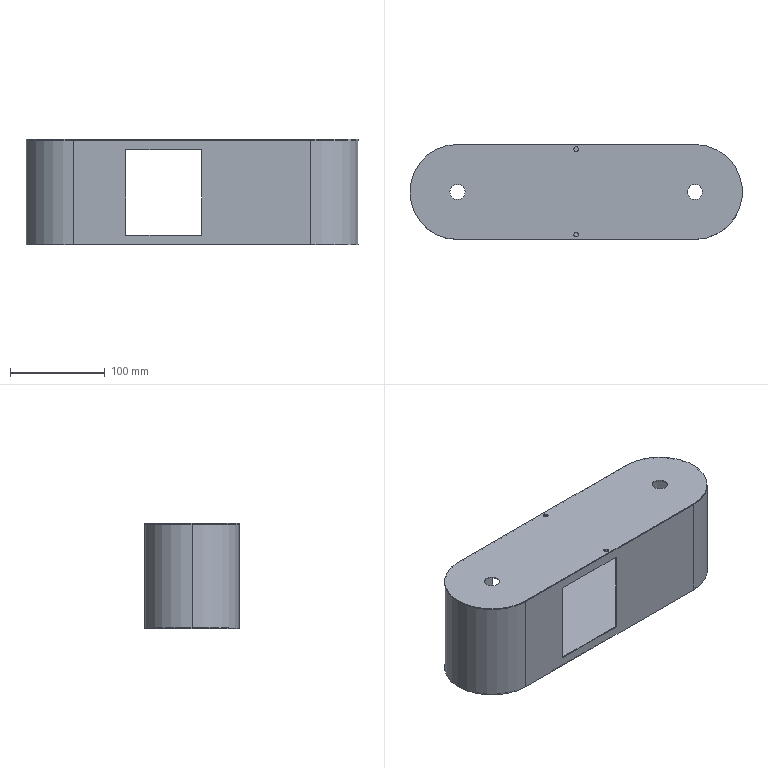Part | SolidWorks | features ICE 5, Extrusion 1, Shell 1 | 2 solids | 40 faces | box 350 x 100 x 111 mm | volume 133465 mm3 | cylinder 21 | plane 19 | commonest cylinder face diameters 16 x8 100 x6 5 x4 98 x3
STEP:
#1=CARTESIAN_POINT('',(122.5,-45.,110.));
#2=VERTEX_POINT('',#1);
#3=CARTESIAN_POINT('',(127.5,-45.,110.));
#4=VERTEX_POINT('',#3);
#5=CARTESIAN_POINT('',(125.,-45.,110.));
#6=DIRECTION('',(0.,0.,1.));
#7=DIRECTION('',(1.,0.,0.));
#8=AXIS2_PLACEMENT_3D('',#5,#6,#7);
#9=CIRCLE('',#8,2.5);
#10=EDGE_CURVE('',#2,#4,#9,.T.);
#11=ORIENTED_EDGE('',*,*,#10,.F.);
#12=CARTESIAN_POINT('',(122.5,-45.,111.));
#13=VERTEX_POINT('',#12);
#14=CARTESIAN_POINT('',(122.5,-45.,108.));
#15=DIRECTION('',(0.,0.,1.));
#16=VECTOR('',#15,1000.);
#17=LINE('',#14,#16);
#18=EDGE_CURVE('',#2,#13,#17,.T.);
#19=ORIENTED_EDGE('',*,*,#18,.T.);
#20=CARTESIAN_POINT('',(127.5,-45.,111.));
#21=VERTEX_POINT('',#20);
#22=CARTESIAN_POINT('',(125.,-45.,111.));
#23=DIRECTION('',(0.,0.,1.));
#24=DIRECTION('',(1.,0.,0.));
#25=AXIS2_PLACEMENT_3D('',#22,#23,#24);
#26=CIRCLE('',#25,2.5);
#27=EDGE_CURVE('',#13,#21,#26,.T.);
#28=ORIENTED_EDGE('',*,*,#27,.T.);
#29=CARTESIAN_POINT('',(127.5,-45.,108.));
#30=DIRECTION('',(0.,0.,1.));
#31=VECTOR('',#30,1000.);
#32=LINE('',#29,#31);
#33=EDGE_CURVE('',#4,#21,#32,.T.);
#34=ORIENTED_EDGE('',*,*,#33,.F.);
#35=EDGE_LOOP('',(#11,#19,#28,#34));
#36=FACE_OUTER_BOUND('',#35,.T.);
#37=CARTESIAN_POINT('',(125.,-45.,108.));
#38=DIRECTION('',(0.,0.,1.));
#39=DIRECTION('',(1.,0.,0.));
#40=AXIS2_PLACEMENT_3D('',#37,#38,#39);
#41=CYLINDRICAL_SURFACE('',#40,2.5);
#42=ADVANCED_FACE('',(#36),#41,.F.);
#43=CARTESIAN_POINT('',(122.5,45.,110.));
#44=VERTEX_POINT('',#43);
#45=CARTESIAN_POINT('',(127.5,45.,110.));
#46=VERTEX_POINT('',#45);
#47=CARTESIAN_POINT('',(125.,45.,110.));
#48=DIRECTION('',(0.,0.,1.));
#49=DIRECTION('',(1.,0.,0.));
#50=AXIS2_PLACEMENT_3D('',#47,#48,#49);
#51=CIRCLE('',#50,2.5);
#52=EDGE_CURVE('',#44,#46,#51,.T.);
#53=ORIENTED_EDGE('',*,*,#52,.F.);
#54=CARTESIAN_POINT('',(122.5,45.,111.));
#55=VERTEX_POINT('',#54);
#56=CARTESIAN_POINT('',(122.5,45.,108.));
#57=DIRECTION('',(0.,0.,1.));
#58=VECTOR('',#57,1000.);
#59=LINE('',#56,#58);
#60=EDGE_CURVE('',#44,#55,#59,.T.);
#61=ORIENTED_EDGE('',*,*,#60,.T.);
#62=CARTESIAN_POINT('',(127.5,45.,111.));
#63=VERTEX_POINT('',#62);
#64=CARTESIAN_POINT('',(125.,45.,111.));
#65=DIRECTION('',(0.,0.,1.));
#66=DIRECTION('',(1.,0.,0.));
#67=AXIS2_PLACEMENT_3D('',#64,#65,#66);
#68=CIRCLE('',#67,2.5);
#69=EDGE_CURVE('',#55,#63,#68,.T.);
#70=ORIENTED_EDGE('',*,*,#69,.T.);
#71=CARTESIAN_POINT('',(127.5,45.,108.));
#72=DIRECTION('',(0.,0.,1.));
#73=VECTOR('',#72,1000.);
#74=LINE('',#71,#73);
#75=EDGE_CURVE('',#46,#63,#74,.T.);
#76=ORIENTED_EDGE('',*,*,#75,.F.);
#77=EDGE_LOOP('',(#53,#61,#70,#76));
#78=FACE_OUTER_BOUND('',#77,.T.);
#79=CARTESIAN_POINT('',(125.,45.,108.));
#80=DIRECTION('',(0.,0.,1.));
#81=DIRECTION('',(1.,0.,0.));
#82=AXIS2_PLACEMENT_3D('',#79,#80,#81);
#83=CYLINDRICAL_SURFACE('',#82,2.5);
#84=ADVANCED_FACE('',(#78),#83,.F.);
#85=CARTESIAN_POINT('',(-8.,0.,110.));
#86=VERTEX_POINT('',#85);
#87=CARTESIAN_POINT('',(8.,0.,110.));
#88=VERTEX_POINT('',#87);
#89=CARTESIAN_POINT('',(0.,0.,110.));
#90=DIRECTION('',(0.,0.,1.));
#91=DIRECTION('',(1.,0.,0.));
#92=AXIS2_PLACEMENT_3D('',#89,#90,#91);
#93=CIRCLE('',#92,8.);
#94=EDGE_CURVE('',#86,#88,#93,.T.);
#95=ORIENTED_EDGE('',*,*,#94,.F.);
#96=CARTESIAN_POINT('',(-8.,0.,111.));
#97=VERTEX_POINT('',#96);
#98=CARTESIAN_POINT('',(-8.,0.,0.));
#99=DIRECTION('',(0.,0.,1.));
#100=VECTOR('',#99,1000.);
#101=LINE('',#98,#100);
#102=EDGE_CURVE('',#86,#97,#101,.T.);
#103=ORIENTED_EDGE('',*,*,#102,.T.);
#104=CARTESIAN_POINT('',(8.,0.,111.));
#105=VERTEX_POINT('',#104);
#106=CARTESIAN_POINT('',(0.,0.,111.));
#107=DIRECTION('',(0.,0.,1.));
#108=DIRECTION('',(1.,0.,0.));
#109=AXIS2_PLACEMENT_3D('',#106,#107,#108);
#110=CIRCLE('',#109,8.);
#111=EDGE_CURVE('',#97,#105,#110,.T.);
#112=ORIENTED_EDGE('',*,*,#111,.T.);
#113=CARTESIAN_POINT('',(8.,0.,0.));
#114=DIRECTION('',(0.,0.,1.));
#115=VECTOR('',#114,1000.);
#116=LINE('',#113,#115);
#117=EDGE_CURVE('',#88,#105,#116,.T.);
#118=ORIENTED_EDGE('',*,*,#117,.F.);
#119=EDGE_LOOP('',(#95,#103,#112,#118));
#120=FACE_OUTER_BOUND('',#119,.T.);
#121=CARTESIAN_POINT('',(0.,0.,0.));
#122=DIRECTION('',(0.,0.,1.));
#123=DIRECTION('',(1.,0.,0.));
#124=AXIS2_PLACEMENT_3D('',#121,#122,#123);
#125=CYLINDRICAL_SURFACE('',#124,8.);
#126=ADVANCED_FACE('',(#120),#125,.F.);
#127=CARTESIAN_POINT('',(242.,0.,110.));
#128=VERTEX_POINT('',#127);
#129=CARTESIAN_POINT('',(258.,0.,110.));
#130=VERTEX_POINT('',#129);
#131=CARTESIAN_POINT('',(250.,0.,110.));
#132=DIRECTION('',(0.,0.,1.));
#133=DIRECTION('',(1.,0.,0.));
#134=AXIS2_PLACEMENT_3D('',#131,#132,#133);
#135=CIRCLE('',#134,8.);
#136=EDGE_CURVE('',#128,#130,#135,.T.);
#137=ORIENTED_EDGE('',*,*,#136,.F.);
#138=CARTESIAN_POINT('',(242.,0.,111.));
#139=VERTEX_POINT('',#138);
#140=CARTESIAN_POINT('',(242.,0.,0.));
#141=DIRECTION('',(0.,0.,1.));
#142=VECTOR('',#141,1000.);
#143=LINE('',#140,#142);
#144=EDGE_CURVE('',#128,#139,#143,.T.);
#145=ORIENTED_EDGE('',*,*,#144,.T.);
#146=CARTESIAN_POINT('',(258.,0.,111.));
#147=VERTEX_POINT('',#146);
#148=CARTESIAN_POINT('',(250.,0.,111.));
#149=DIRECTION('',(0.,0.,1.));
#150=DIRECTION('',(1.,0.,0.));
#151=AXIS2_PLACEMENT_3D('',#148,#149,#150);
#152=CIRCLE('',#151,8.);
#153=EDGE_CURVE('',#139,#147,#152,.T.);
#154=ORIENTED_EDGE('',*,*,#153,.T.);
#155=CARTESIAN_POINT('',(258.,0.,0.));
#156=DIRECTION('',(0.,0.,1.));
#157=VECTOR('',#156,1000.);
#158=LINE('',#155,#157);
#159=EDGE_CURVE('',#130,#147,#158,.T.);
#160=ORIENTED_EDGE('',*,*,#159,.F.);
#161=EDGE_LOOP('',(#137,#145,#154,#160));
#162=FACE_OUTER_BOUND('',#161,.T.);
#163=CARTESIAN_POINT('',(250.,0.,0.));
#164=DIRECTION('',(0.,0.,1.));
#165=DIRECTION('',(1.,0.,0.));
#166=AXIS2_PLACEMENT_3D('',#163,#164,#165);
#167=CYLINDRICAL_SURFACE('',#166,8.);
#168=ADVANCED_FACE('',(#162),#167,.F.);
#169=CARTESIAN_POINT('',(-50.,0.,111.));
#170=VERTEX_POINT('',#169);
#171=CARTESIAN_POINT('',(0.,-50.,111.));
#172=VERTEX_POINT('',#171);
#173=CARTESIAN_POINT('',(0.,0.,111.));
#174=DIRECTION('',(0.,0.,1.));
#175=DIRECTION('',(1.,0.,0.));
#176=AXIS2_PLACEMENT_3D('',#173,#174,#175);
#177=CIRCLE('',#176,50.);
#178=EDGE_CURVE('',#170,#172,#177,.T.);
#179=ORIENTED_EDGE('',*,*,#178,.F.);
#180=CARTESIAN_POINT('',(-50.,0.,110.));
#181=VERTEX_POINT('',#180);
#182=CARTESIAN_POINT('',(-50.,0.,111.));
#183=DIRECTION('',(0.,0.,-1.));
#184=VECTOR('',#183,1000.);
#185=LINE('',#182,#184);
#186=EDGE_CURVE('',#170,#181,#185,.T.);
#187=ORIENTED_EDGE('',*,*,#186,.T.);
#188=CARTESIAN_POINT('',(0.,-50.,110.));
#189=VERTEX_POINT('',#188);
#190=CARTESIAN_POINT('',(0.,0.,110.));
#191=DIRECTION('',(0.,0.,1.));
#192=DIRECTION('',(1.,0.,0.));
#193=AXIS2_PLACEMENT_3D('',#190,#191,#192);
#194=CIRCLE('',#193,50.);
#195=EDGE_CURVE('',#181,#189,#194,.T.);
#196=ORIENTED_EDGE('',*,*,#195,.T.);
#197=CARTESIAN_POINT('',(0.,-50.,111.));
#198=DIRECTION('',(0.,0.,-1.));
#199=VECTOR('',#198,1000.);
#200=LINE('',#197,#199);
#201=EDGE_CURVE('',#172,#189,#200,.T.);
#202=ORIENTED_EDGE('',*,*,#201,.F.);
#203=EDGE_LOOP('',(#179,#187,#196,#202));
#204=FACE_OUTER_BOUND('',#203,.T.);
#205=CARTESIAN_POINT('',(0.,0.,111.));
#206=DIRECTION('',(0.,0.,-1.));
#207=DIRECTION('',(-1.,0.,0.));
#208=AXIS2_PLACEMENT_3D('',#205,#206,#207);
#209=CYLINDRICAL_SURFACE('',#208,50.);
#210=ADVANCED_FACE('',(#204),#209,.T.);
#211=CARTESIAN_POINT('',(250.,-50.,110.));
#212=VERTEX_POINT('',#211);
#213=CARTESIAN_POINT('',(250.,50.,110.));
#214=VERTEX_POINT('',#213);
#215=CARTESIAN_POINT('',(250.,0.,110.));
#216=DIRECTION('',(0.,0.,1.));
#217=DIRECTION('',(1.,0.,0.));
#218=AXIS2_PLACEMENT_3D('',#215,#216,#217);
#219=CIRCLE('',#218,50.);
#220=EDGE_CURVE('',#212,#214,#219,.T.);
#221=ORIENTED_EDGE('',*,*,#220,.T.);
#222=CARTESIAN_POINT('',(250.,50.,111.));
#223=VERTEX_POINT('',#222);
#224=CARTESIAN_POINT('',(250.,50.,111.));
#225=DIRECTION('',(0.,0.,-1.));
#226=VECTOR('',#225,1000.);
#227=LINE('',#224,#226);
#228=EDGE_CURVE('',#223,#214,#227,.T.);
#229=ORIENTED_EDGE('',*,*,#228,.F.);
#230=CARTESIAN_POINT('',(250.,-50.,111.));
#231=VERTEX_POINT('',#230);
#232=CARTESIAN_POINT('',(250.,0.,111.));
#233=DIRECTION('',(0.,0.,1.));
#234=DIRECTION('',(1.,0.,0.));
#235=AXIS2_PLACEMENT_3D('',#232,#233,#234);
#236=CIRCLE('',#235,50.);
#237=EDGE_CURVE('',#231,#223,#236,.T.);
#238=ORIENTED_EDGE('',*,*,#237,.F.);
#239=CARTESIAN_POINT('',(250.,-50.,111.));
#240=DIRECTION('',(0.,0.,-1.));
#241=VECTOR('',#240,1000.);
#242=LINE('',#239,#241);
#243=EDGE_CURVE('',#231,#212,#242,.T.);
#244=ORIENTED_EDGE('',*,*,#243,.T.);
#245=EDGE_LOOP('',(#221,#229,#238,#244));
#246=FACE_OUTER_BOUND('',#245,.T.);
#247=CARTESIAN_POINT('',(250.,0.,111.));
#248=DIRECTION('',(0.,0.,-1.));
#249=DIRECTION('',(-1.,0.,0.));
#250=AXIS2_PLACEMENT_3D('',#247,#248,#249);
#251=CYLINDRICAL_SURFACE('',#250,50.);
#252=ADVANCED_FACE('',(#246),#251,.T.);
#253=CARTESIAN_POINT('',(0.,50.,110.));
#254=VERTEX_POINT('',#253);
#255=CARTESIAN_POINT('',(250.,50.,110.));
#256=DIRECTION('',(-1.,0.,0.));
#257=VECTOR('',#256,1000.);
#258=LINE('',#255,#257);
#259=EDGE_CURVE('',#214,#254,#258,.T.);
#260=ORIENTED_EDGE('',*,*,#259,.T.);
#261=CARTESIAN_POINT('',(0.,50.,111.));
#262=VERTEX_POINT('',#261);
#263=CARTESIAN_POINT('',(0.,50.,111.));
#264=DIRECTION('',(0.,0.,-1.));
#265=VECTOR('',#264,1000.);
#266=LINE('',#263,#265);
#267=EDGE_CURVE('',#262,#254,#266,.T.);
#268=ORIENTED_EDGE('',*,*,#267,.F.);
#269=CARTESIAN_POINT('',(250.,50.,111.));
#270=DIRECTION('',(-1.,0.,0.));
#271=VECTOR('',#270,1000.);
#272=LINE('',#269,#271);
#273=EDGE_CURVE('',#223,#262,#272,.T.);
#274=ORIENTED_EDGE('',*,*,#273,.F.);
#275=ORIENTED_EDGE('',*,*,#228,.T.);
#276=EDGE_LOOP('',(#260,#268,#274,#275));
#277=FACE_OUTER_BOUND('',#276,.T.);
#278=CARTESIAN_POINT('',(250.,50.,111.));
#279=DIRECTION('',(0.,-1.,0.));
#280=DIRECTION('',(0.,0.,-1.));
#281=AXIS2_PLACEMENT_3D('',#278,#279,#280);
#282=PLANE('',#281);
#283=ADVANCED_FACE('',(#277),#282,.F.);
#284=ORIENTED_EDGE('',*,*,#186,.F.);
#285=CARTESIAN_POINT('',(0.,0.,111.));
#286=DIRECTION('',(0.,0.,1.));
#287=DIRECTION('',(1.,0.,0.));
#288=AXIS2_PLACEMENT_3D('',#285,#286,#287);
#289=CIRCLE('',#288,50.);
#290=EDGE_CURVE('',#262,#170,#289,.T.);
#291=ORIENTED_EDGE('',*,*,#290,.F.);
#292=ORIENTED_EDGE('',*,*,#267,.T.);
#293=CARTESIAN_POINT('',(0.,0.,110.));
#294=DIRECTION('',(0.,0.,1.));
#295=DIRECTION('',(1.,0.,0.));
#296=AXIS2_PLACEMENT_3D('',#293,#294,#295);
#297=CIRCLE('',#296,50.);
#298=EDGE_CURVE('',#254,#181,#297,.T.);
#299=ORIENTED_EDGE('',*,*,#298,.T.);
#300=EDGE_LOOP('',(#284,#291,#292,#299));
#301=FACE_OUTER_BOUND('',#300,.T.);
#302=CARTESIAN_POINT('',(0.,0.,111.));
#303=DIRECTION('',(0.,0.,-1.));
#304=DIRECTION('',(-1.,0.,0.));
#305=AXIS2_PLACEMENT_3D('',#302,#303,#304);
#306=CYLINDRICAL_SURFACE('',#305,50.);
#307=ADVANCED_FACE('',(#301),#306,.T.);
#308=CARTESIAN_POINT('',(0.,-50.,110.));
#309=DIRECTION('',(1.,0.,0.));
#310=VECTOR('',#309,1000.);
#311=LINE('',#308,#310);
#312=EDGE_CURVE('',#189,#212,#311,.T.);
#313=ORIENTED_EDGE('',*,*,#312,.T.);
#314=ORIENTED_EDGE('',*,*,#243,.F.);
#315=CARTESIAN_POINT('',(0.,-50.,111.));
#316=DIRECTION('',(1.,0.,0.));
#317=VECTOR('',#316,1000.);
#318=LINE('',#315,#317);
#319=EDGE_CURVE('',#172,#231,#318,.T.);
#320=ORIENTED_EDGE('',*,*,#319,.F.);
#321=ORIENTED_EDGE('',*,*,#201,.T.);
#322=EDGE_LOOP('',(#313,#314,#320,#321));
#323=FACE_OUTER_BOUND('',#322,.T.);
#324=CARTESIAN_POINT('',(0.,-50.,111.));
#325=DIRECTION('',(0.,1.,0.));
#326=DIRECTION('',(0.,0.,1.));
#327=AXIS2_PLACEMENT_3D('',#324,#325,#326);
#328=PLANE('',#327);
#329=ADVANCED_FACE('',(#323),#328,.F.);
#330=CARTESIAN_POINT('',(125.,-45.,111.));
#331=DIRECTION('',(0.,0.,1.));
#332=DIRECTION('',(1.,0.,0.));
#333=AXIS2_PLACEMENT_3D('',#330,#331,#332);
#334=CIRCLE('',#333,2.5);
#335=EDGE_CURVE('',#21,#13,#334,.T.);
#336=ORIENTED_EDGE('',*,*,#335,.F.);
#337=ORIENTED_EDGE('',*,*,#27,.F.);
#338=EDGE_LOOP('',(#336,#337));
#339=FACE_BOUND('',#338,.T.);
#340=CARTESIAN_POINT('',(125.,45.,111.));
#341=DIRECTION('',(0.,0.,1.));
#342=DIRECTION('',(1.,0.,0.));
#343=AXIS2_PLACEMENT_3D('',#340,#341,#342);
#344=CIRCLE('',#343,2.5);
#345=EDGE_CURVE('',#63,#55,#344,.T.);
#346=ORIENTED_EDGE('',*,*,#345,.F.);
#347=ORIENTED_EDGE('',*,*,#69,.F.);
#348=EDGE_LOOP('',(#346,#347));
#349=FACE_BOUND('',#348,.T.);
#350=CARTESIAN_POINT('',(0.,0.,111.));
#351=DIRECTION('',(0.,0.,1.));
#352=DIRECTION('',(1.,0.,0.));
#353=AXIS2_PLACEMENT_3D('',#350,#351,#352);
#354=CIRCLE('',#353,8.);
#355=EDGE_CURVE('',#105,#97,#354,.T.);
#356=ORIENTED_EDGE('',*,*,#355,.F.);
#357=ORIENTED_EDGE('',*,*,#111,.F.);
#358=EDGE_LOOP('',(#356,#357));
#359=FACE_BOUND('',#358,.T.);
#360=CARTESIAN_POINT('',(250.,0.,111.));
#361=DIRECTION('',(0.,0.,1.));
#362=DIRECTION('',(1.,0.,0.));
#363=AXIS2_PLACEMENT_3D('',#360,#361,#362);
#364=CIRCLE('',#363,8.);
#365=EDGE_CURVE('',#147,#139,#364,.T.);
#366=ORIENTED_EDGE('',*,*,#365,.F.);
#367=ORIENTED_EDGE('',*,*,#153,.F.);
#368=EDGE_LOOP('',(#366,#367));
#369=FACE_BOUND('',#368,.T.);
#370=ORIENTED_EDGE('',*,*,#237,.T.);
#371=ORIENTED_EDGE('',*,*,#273,.T.);
#372=ORIENTED_EDGE('',*,*,#290,.T.);
#373=ORIENTED_EDGE('',*,*,#178,.T.);
#374=ORIENTED_EDGE('',*,*,#319,.T.);
#375=EDGE_LOOP('',(#370,#371,#372,#373,#374));
#376=FACE_OUTER_BOUND('',#375,.T.);
#377=CARTESIAN_POINT('',(250.,0.,111.));
#378=DIRECTION('',(0.,0.,1.));
#379=DIRECTION('',(1.,0.,0.));
#380=AXIS2_PLACEMENT_3D('',#377,#378,#379);
#381=PLANE('',#380);
#382=ADVANCED_FACE('',(#339,#349,#359,#369,#376),#381,.T.);
#383=CARTESIAN_POINT('',(125.,-45.,110.));
#384=DIRECTION('',(0.,0.,1.));
#385=DIRECTION('',(1.,0.,0.));
#386=AXIS2_PLACEMENT_3D('',#383,#384,#385);
#387=CIRCLE('',#386,2.5);
#388=EDGE_CURVE('',#4,#2,#387,.T.);
#389=ORIENTED_EDGE('',*,*,#388,.T.);
#390=ORIENTED_EDGE('',*,*,#10,.T.);
#391=EDGE_LOOP('',(#389,#390));
#392=FACE_BOUND('',#391,.T.);
#393=CARTESIAN_POINT('',(125.,45.,110.));
#394=DIRECTION('',(0.,0.,1.));
#395=DIRECTION('',(1.,0.,0.));
#396=AXIS2_PLACEMENT_3D('',#393,#394,#395);
#397=CIRCLE('',#396,2.5);
#398=EDGE_CURVE('',#46,#44,#397,.T.);
#399=ORIENTED_EDGE('',*,*,#398,.T.);
#400=ORIENTED_EDGE('',*,*,#52,.T.);
#401=EDGE_LOOP('',(#399,#400));
#402=FACE_BOUND('',#401,.T.);
#403=CARTESIAN_POINT('',(0.,0.,110.));
#404=DIRECTION('',(0.,0.,1.));
#405=DIRECTION('',(1.,0.,0.));
#406=AXIS2_PLACEMENT_3D('',#403,#404,#405);
#407=CIRCLE('',#406,8.);
#408=EDGE_CURVE('',#88,#86,#407,.T.);
#409=ORIENTED_EDGE('',*,*,#408,.T.);
#410=ORIENTED_EDGE('',*,*,#94,.T.);
#411=EDGE_LOOP('',(#409,#410));
#412=FACE_BOUND('',#411,.T.);
#413=CARTESIAN_POINT('',(250.,0.,110.));
#414=DIRECTION('',(0.,0.,1.));
#415=DIRECTION('',(1.,0.,0.));
#416=AXIS2_PLACEMENT_3D('',#413,#414,#415);
#417=CIRCLE('',#416,8.);
#418=EDGE_CURVE('',#130,#128,#417,.T.);
#419=ORIENTED_EDGE('',*,*,#418,.T.);
#420=ORIENTED_EDGE('',*,*,#136,.T.);
#421=EDGE_LOOP('',(#419,#420));
#422=FACE_BOUND('',#421,.T.);
#423=ORIENTED_EDGE('',*,*,#220,.F.);
#424=ORIENTED_EDGE('',*,*,#312,.F.);
#425=ORIENTED_EDGE('',*,*,#195,.F.);
#426=ORIENTED_EDGE('',*,*,#298,.F.);
#427=ORIENTED_EDGE('',*,*,#259,.F.);
#428=EDGE_LOOP('',(#423,#424,#425,#426,#427));
#429=FACE_OUTER_BOUND('',#428,.T.);
#430=CARTESIAN_POINT('',(250.,0.,110.));
#431=DIRECTION('',(0.,0.,1.));
#432=DIRECTION('',(1.,0.,0.));
#433=AXIS2_PLACEMENT_3D('',#430,#431,#432);
#434=PLANE('',#433);
#435=ADVANCED_FACE('',(#392,#402,#412,#422,#429),#434,.F.);
#436=ORIENTED_EDGE('',*,*,#144,.F.);
#437=ORIENTED_EDGE('',*,*,#418,.F.);
#438=ORIENTED_EDGE('',*,*,#159,.T.);
#439=ORIENTED_EDGE('',*,*,#365,.T.);
#440=EDGE_LOOP('',(#436,#437,#438,#439));
#441=FACE_OUTER_BOUND('',#440,.T.);
#442=CARTESIAN_POINT('',(250.,0.,0.));
#443=DIRECTION('',(0.,0.,1.));
#444=DIRECTION('',(1.,0.,0.));
#445=AXIS2_PLACEMENT_3D('',#442,#443,#444);
#446=CYLINDRICAL_SURFACE('',#445,8.);
#447=ADVANCED_FACE('',(#441),#446,.F.);
#448=ORIENTED_EDGE('',*,*,#102,.F.);
#449=ORIENTED_EDGE('',*,*,#408,.F.);
#450=ORIENTED_EDGE('',*,*,#117,.T.);
#451=ORIENTED_EDGE('',*,*,#355,.T.);
#452=EDGE_LOOP('',(#448,#449,#450,#451));
#453=FACE_OUTER_BOUND('',#452,.T.);
#454=CARTESIAN_POINT('',(0.,0.,0.));
#455=DIRECTION('',(0.,0.,1.));
#456=DIRECTION('',(1.,0.,0.));
#457=AXIS2_PLACEMENT_3D('',#454,#455,#456);
#458=CYLINDRICAL_SURFACE('',#457,8.);
#459=ADVANCED_FACE('',(#453),#458,.F.);
#460=ORIENTED_EDGE('',*,*,#60,.F.);
#461=ORIENTED_EDGE('',*,*,#398,.F.);
#462=ORIENTED_EDGE('',*,*,#75,.T.);
#463=ORIENTED_EDGE('',*,*,#345,.T.);
#464=EDGE_LOOP('',(#460,#461,#462,#463));
#465=FACE_OUTER_BOUND('',#464,.T.);
#466=CARTESIAN_POINT('',(125.,45.,108.));
#467=DIRECTION('',(0.,0.,1.));
#468=DIRECTION('',(1.,0.,0.));
#469=AXIS2_PLACEMENT_3D('',#466,#467,#468);
#470=CYLINDRICAL_SURFACE('',#469,2.5);
#471=ADVANCED_FACE('',(#465),#470,.F.);
#472=ORIENTED_EDGE('',*,*,#18,.F.);
#473=ORIENTED_EDGE('',*,*,#388,.F.);
#474=ORIENTED_EDGE('',*,*,#33,.T.);
#475=ORIENTED_EDGE('',*,*,#335,.T.);
#476=EDGE_LOOP('',(#472,#473,#474,#475));
#477=FACE_OUTER_BOUND('',#476,.T.);
#478=CARTESIAN_POINT('',(125.,-45.,108.));
#479=DIRECTION('',(0.,0.,1.));
#480=DIRECTION('',(1.,0.,0.));
#481=AXIS2_PLACEMENT_3D('',#478,#479,#480);
#482=CYLINDRICAL_SURFACE('',#481,2.5);
#483=ADVANCED_FACE('',(#477),#482,.F.);
#484=CLOSED_SHELL('',(#42,#84,#126,#168,#210,#252,#283,#307,#329,#382,#435,#447,#459,#471,#483));
#485=MANIFOLD_SOLID_BREP('',#484);
#486=CARTESIAN_POINT('',(-8.,0.,0.));
#487=VERTEX_POINT('',#486);
#488=CARTESIAN_POINT('',(8.,0.,0.));
#489=VERTEX_POINT('',#488);
#490=CARTESIAN_POINT('',(0.,0.,0.));
#491=DIRECTION('',(0.,0.,1.));
#492=DIRECTION('',(1.,0.,0.));
#493=AXIS2_PLACEMENT_3D('',#490,#491,#492);
#494=CIRCLE('',#493,8.);
#495=EDGE_CURVE('',#487,#489,#494,.T.);
#496=ORIENTED_EDGE('',*,*,#495,.F.);
#497=CARTESIAN_POINT('',(-8.,0.,1.));
#498=VERTEX_POINT('',#497);
#499=CARTESIAN_POINT('',(-8.,0.,0.));
#500=DIRECTION('',(0.,0.,1.));
#501=VECTOR('',#500,1000.);
#502=LINE('',#499,#501);
#503=EDGE_CURVE('',#487,#498,#502,.T.);
#504=ORIENTED_EDGE('',*,*,#503,.T.);
#505=CARTESIAN_POINT('',(8.,0.,1.));
#506=VERTEX_POINT('',#505);
#507=CARTESIAN_POINT('',(0.,0.,1.));
#508=DIRECTION('',(0.,0.,1.));
#509=DIRECTION('',(1.,0.,0.));
#510=AXIS2_PLACEMENT_3D('',#507,#508,#509);
#511=CIRCLE('',#510,8.);
#512=EDGE_CURVE('',#498,#506,#511,.T.);
#513=ORIENTED_EDGE('',*,*,#512,.T.);
#514=CARTESIAN_POINT('',(8.,0.,0.));
#515=DIRECTION('',(0.,0.,1.));
#516=VECTOR('',#515,1000.);
#517=LINE('',#514,#516);
#518=EDGE_CURVE('',#489,#506,#517,.T.);
#519=ORIENTED_EDGE('',*,*,#518,.F.);
#520=EDGE_LOOP('',(#496,#504,#513,#519));
#521=FACE_OUTER_BOUND('',#520,.T.);
#522=CARTESIAN_POINT('',(0.,0.,0.));
#523=DIRECTION('',(0.,0.,1.));
#524=DIRECTION('',(1.,0.,0.));
#525=AXIS2_PLACEMENT_3D('',#522,#523,#524);
#526=CYLINDRICAL_SURFACE('',#525,8.);
#527=ADVANCED_FACE('',(#521),#526,.F.);
#528=CARTESIAN_POINT('',(242.,0.,0.));
#529=VERTEX_POINT('',#528);
#530=CARTESIAN_POINT('',(258.,0.,0.));
#531=VERTEX_POINT('',#530);
#532=CARTESIAN_POINT('',(250.,0.,0.));
#533=DIRECTION('',(0.,0.,1.));
#534=DIRECTION('',(1.,0.,0.));
#535=AXIS2_PLACEMENT_3D('',#532,#533,#534);
#536=CIRCLE('',#535,8.);
#537=EDGE_CURVE('',#529,#531,#536,.T.);
#538=ORIENTED_EDGE('',*,*,#537,.F.);
#539=CARTESIAN_POINT('',(242.,0.,1.));
#540=VERTEX_POINT('',#539);
#541=CARTESIAN_POINT('',(242.,0.,0.));
#542=DIRECTION('',(0.,0.,1.));
#543=VECTOR('',#542,1000.);
#544=LINE('',#541,#543);
#545=EDGE_CURVE('',#529,#540,#544,.T.);
#546=ORIENTED_EDGE('',*,*,#545,.T.);
#547=CARTESIAN_POINT('',(258.,0.,1.));
#548=VERTEX_POINT('',#547);
#549=CARTESIAN_POINT('',(250.,0.,1.));
#550=DIRECTION('',(0.,0.,1.));
#551=DIRECTION('',(1.,0.,0.));
#552=AXIS2_PLACEMENT_3D('',#549,#550,#551);
#553=CIRCLE('',#552,8.);
#554=EDGE_CURVE('',#540,#548,#553,.T.);
#555=ORIENTED_EDGE('',*,*,#554,.T.);
#556=CARTESIAN_POINT('',(258.,0.,0.));
#557=DIRECTION('',(0.,0.,1.));
#558=VECTOR('',#557,1000.);
#559=LINE('',#556,#558);
#560=EDGE_CURVE('',#531,#548,#559,.T.);
#561=ORIENTED_EDGE('',*,*,#560,.F.);
#562=EDGE_LOOP('',(#538,#546,#555,#561));
#563=FACE_OUTER_BOUND('',#562,.T.);
#564=CARTESIAN_POINT('',(250.,0.,0.));
#565=DIRECTION('',(0.,0.,1.));
#566=DIRECTION('',(1.,0.,0.));
#567=AXIS2_PLACEMENT_3D('',#564,#565,#566);
#568=CYLINDRICAL_SURFACE('',#567,8.);
#569=ADVANCED_FACE('',(#563),#568,.F.);
#570=CARTESIAN_POINT('',(0.,49.,110.));
#571=VERTEX_POINT('',#570);
#572=CARTESIAN_POINT('',(-49.,0.,110.));
#573=VERTEX_POINT('',#572);
#574=CARTESIAN_POINT('',(0.,0.,110.));
#575=DIRECTION('',(0.,0.,1.));
#576=DIRECTION('',(1.,0.,0.));
#577=AXIS2_PLACEMENT_3D('',#574,#575,#576);
#578=CIRCLE('',#577,49.);
#579=EDGE_CURVE('',#571,#573,#578,.T.);
#580=ORIENTED_EDGE('',*,*,#579,.T.);
#581=CARTESIAN_POINT('',(-49.,0.,1.));
#582=VERTEX_POINT('',#581);
#583=CARTESIAN_POINT('',(-49.,0.,110.));
#584=DIRECTION('',(0.,0.,-1.));
#585=VECTOR('',#584,1000.);
#586=LINE('',#583,#585);
#587=EDGE_CURVE('',#573,#582,#586,.T.);
#588=ORIENTED_EDGE('',*,*,#587,.T.);
#589=CARTESIAN_POINT('',(0.,49.,1.));
#590=VERTEX_POINT('',#589);
#591=CARTESIAN_POINT('',(0.,0.,1.));
#592=DIRECTION('',(0.,0.,1.));
#593=DIRECTION('',(1.,0.,0.));
#594=AXIS2_PLACEMENT_3D('',#591,#592,#593);
#595=CIRCLE('',#594,49.);
#596=EDGE_CURVE('',#590,#582,#595,.T.);
#597=ORIENTED_EDGE('',*,*,#596,.F.);
#598=CARTESIAN_POINT('',(0.,49.,110.));
#599=DIRECTION('',(0.,0.,-1.));
#600=VECTOR('',#599,1000.);
#601=LINE('',#598,#600);
#602=EDGE_CURVE('',#571,#590,#601,.T.);
#603=ORIENTED_EDGE('',*,*,#602,.F.);
#604=EDGE_LOOP('',(#580,#588,#597,#603));
#605=FACE_OUTER_BOUND('',#604,.T.);
#606=CARTESIAN_POINT('',(0.,0.,110.));
#607=DIRECTION('',(0.,0.,-1.));
#608=DIRECTION('',(-1.,0.,0.));
#609=AXIS2_PLACEMENT_3D('',#606,#607,#608);
#610=CYLINDRICAL_SURFACE('',#609,49.);
#611=ADVANCED_FACE('',(#605),#610,.F.);
#612=CARTESIAN_POINT('',(-50.,0.,110.));
#613=VERTEX_POINT('',#612);
#614=CARTESIAN_POINT('',(0.,-50.,110.));
#615=VERTEX_POINT('',#614);
#616=CARTESIAN_POINT('',(0.,0.,110.));
#617=DIRECTION('',(0.,0.,1.));
#618=DIRECTION('',(1.,0.,0.));
#619=AXIS2_PLACEMENT_3D('',#616,#617,#618);
#620=CIRCLE('',#619,50.);
#621=EDGE_CURVE('',#613,#615,#620,.T.);
#622=ORIENTED_EDGE('',*,*,#621,.F.);
#623=CARTESIAN_POINT('',(-50.,0.,0.));
#624=VERTEX_POINT('',#623);
#625=CARTESIAN_POINT('',(-50.,0.,110.));
#626=DIRECTION('',(0.,0.,-1.));
#627=VECTOR('',#626,1000.);
#628=LINE('',#625,#627);
#629=EDGE_CURVE('',#613,#624,#628,.T.);
#630=ORIENTED_EDGE('',*,*,#629,.T.);
#631=CARTESIAN_POINT('',(0.,-50.,0.));
#632=VERTEX_POINT('',#631);
#633=CARTESIAN_POINT('',(0.,0.,0.));
#634=DIRECTION('',(0.,0.,1.));
#635=DIRECTION('',(1.,0.,0.));
#636=AXIS2_PLACEMENT_3D('',#633,#634,#635);
#637=CIRCLE('',#636,50.);
#638=EDGE_CURVE('',#624,#632,#637,.T.);
#639=ORIENTED_EDGE('',*,*,#638,.T.);
#640=CARTESIAN_POINT('',(0.,-50.,110.));
#641=DIRECTION('',(0.,0.,-1.));
#642=VECTOR('',#641,1000.);
#643=LINE('',#640,#642);
#644=EDGE_CURVE('',#615,#632,#643,.T.);
#645=ORIENTED_EDGE('',*,*,#644,.F.);
#646=EDGE_LOOP('',(#622,#630,#639,#645));
#647=FACE_OUTER_BOUND('',#646,.T.);
#648=CARTESIAN_POINT('',(0.,0.,110.));
#649=DIRECTION('',(0.,0.,-1.));
#650=DIRECTION('',(-1.,0.,0.));
#651=AXIS2_PLACEMENT_3D('',#648,#649,#650);
#652=CYLINDRICAL_SURFACE('',#651,50.);
#653=ADVANCED_FACE('',(#647),#652,.T.);
#654=ORIENTED_EDGE('',*,*,#629,.F.);
#655=CARTESIAN_POINT('',(0.,50.,110.));
#656=VERTEX_POINT('',#655);
#657=CARTESIAN_POINT('',(0.,0.,110.));
#658=DIRECTION('',(0.,0.,1.));
#659=DIRECTION('',(1.,0.,0.));
#660=AXIS2_PLACEMENT_3D('',#657,#658,#659);
#661=CIRCLE('',#660,50.);
#662=EDGE_CURVE('',#656,#613,#661,.T.);
#663=ORIENTED_EDGE('',*,*,#662,.F.);
#664=CARTESIAN_POINT('',(0.,50.,0.));
#665=VERTEX_POINT('',#664);
#666=CARTESIAN_POINT('',(0.,50.,110.));
#667=DIRECTION('',(0.,0.,-1.));
#668=VECTOR('',#667,1000.);
#669=LINE('',#666,#668);
#670=EDGE_CURVE('',#656,#665,#669,.T.);
#671=ORIENTED_EDGE('',*,*,#670,.T.);
#672=CARTESIAN_POINT('',(0.,0.,0.));
#673=DIRECTION('',(0.,0.,1.));
#674=DIRECTION('',(1.,0.,0.));
#675=AXIS2_PLACEMENT_3D('',#672,#673,#674);
#676=CIRCLE('',#675,50.);
#677=EDGE_CURVE('',#665,#624,#676,.T.);
#678=ORIENTED_EDGE('',*,*,#677,.T.);
#679=EDGE_LOOP('',(#654,#663,#671,#678));
#680=FACE_OUTER_BOUND('',#679,.T.);
#681=CARTESIAN_POINT('',(0.,0.,110.));
#682=DIRECTION('',(0.,0.,-1.));
#683=DIRECTION('',(-1.,0.,0.));
#684=AXIS2_PLACEMENT_3D('',#681,#682,#683);
#685=CYLINDRICAL_SURFACE('',#684,50.);
#686=ADVANCED_FACE('',(#680),#685,.T.);
#687=CARTESIAN_POINT('',(135.,-50.,100.));
#688=VERTEX_POINT('',#687);
#689=CARTESIAN_POINT('',(55.,-50.,100.));
#690=VERTEX_POINT('',#689);
#691=CARTESIAN_POINT('',(55.,-50.,100.));
#692=DIRECTION('',(-1.,0.,0.));
#693=VECTOR('',#692,1000.);
#694=LINE('',#691,#693);
#695=EDGE_CURVE('',#688,#690,#694,.T.);
#696=ORIENTED_EDGE('',*,*,#695,.F.);
#697=CARTESIAN_POINT('',(135.,-50.,10.));
#698=VERTEX_POINT('',#697);
#699=CARTESIAN_POINT('',(135.,-50.,10.));
#700=DIRECTION('',(0.,0.,1.));
#701=VECTOR('',#700,1000.);
#702=LINE('',#699,#701);
#703=EDGE_CURVE('',#698,#688,#702,.T.);
#704=ORIENTED_EDGE('',*,*,#703,.F.);
#705=CARTESIAN_POINT('',(55.,-50.,10.));
#706=VERTEX_POINT('',#705);
#707=CARTESIAN_POINT('',(55.,-50.,10.));
#708=DIRECTION('',(1.,0.,0.));
#709=VECTOR('',#708,1000.);
#710=LINE('',#707,#709);
#711=EDGE_CURVE('',#706,#698,#710,.T.);
#712=ORIENTED_EDGE('',*,*,#711,.F.);
#713=CARTESIAN_POINT('',(55.,-50.,10.));
#714=DIRECTION('',(0.,0.,-1.));
#715=VECTOR('',#714,1000.);
#716=LINE('',#713,#715);
#717=EDGE_CURVE('',#690,#706,#716,.T.);
#718=ORIENTED_EDGE('',*,*,#717,.F.);
#719=EDGE_LOOP('',(#696,#704,#712,#718));
#720=FACE_BOUND('',#719,.T.);
#721=CARTESIAN_POINT('',(250.,-50.,0.));
#722=VERTEX_POINT('',#721);
#723=CARTESIAN_POINT('',(0.,-50.,0.));
#724=DIRECTION('',(1.,0.,0.));
#725=VECTOR('',#724,1000.);
#726=LINE('',#723,#725);
#727=EDGE_CURVE('',#632,#722,#726,.T.);
#728=ORIENTED_EDGE('',*,*,#727,.T.);
#729=CARTESIAN_POINT('',(250.,-50.,110.));
#730=VERTEX_POINT('',#729);
#731=CARTESIAN_POINT('',(250.,-50.,110.));
#732=DIRECTION('',(0.,0.,-1.));
#733=VECTOR('',#732,1000.);
#734=LINE('',#731,#733);
#735=EDGE_CURVE('',#730,#722,#734,.T.);
#736=ORIENTED_EDGE('',*,*,#735,.F.);
#737=CARTESIAN_POINT('',(0.,-50.,110.));
#738=DIRECTION('',(1.,0.,0.));
#739=VECTOR('',#738,1000.);
#740=LINE('',#737,#739);
#741=EDGE_CURVE('',#615,#730,#740,.T.);
#742=ORIENTED_EDGE('',*,*,#741,.F.);
#743=ORIENTED_EDGE('',*,*,#644,.T.);
#744=EDGE_LOOP('',(#728,#736,#742,#743));
#745=FACE_OUTER_BOUND('',#744,.T.);
#746=CARTESIAN_POINT('',(0.,-50.,110.));
#747=DIRECTION('',(0.,1.,0.));
#748=DIRECTION('',(0.,0.,1.));
#749=AXIS2_PLACEMENT_3D('',#746,#747,#748);
#750=PLANE('',#749);
#751=ADVANCED_FACE('',(#720,#745),#750,.F.);
#752=CARTESIAN_POINT('',(250.,50.,0.));
#753=VERTEX_POINT('',#752);
#754=CARTESIAN_POINT('',(250.,0.,0.));
#755=DIRECTION('',(0.,0.,1.));
#756=DIRECTION('',(1.,0.,0.));
#757=AXIS2_PLACEMENT_3D('',#754,#755,#756);
#758=CIRCLE('',#757,50.);
#759=EDGE_CURVE('',#722,#753,#758,.T.);
#760=ORIENTED_EDGE('',*,*,#759,.T.);
#761=CARTESIAN_POINT('',(250.,50.,110.));
#762=VERTEX_POINT('',#761);
#763=CARTESIAN_POINT('',(250.,50.,110.));
#764=DIRECTION('',(0.,0.,-1.));
#765=VECTOR('',#764,1000.);
#766=LINE('',#763,#765);
#767=EDGE_CURVE('',#762,#753,#766,.T.);
#768=ORIENTED_EDGE('',*,*,#767,.F.);
#769=CARTESIAN_POINT('',(250.,0.,110.));
#770=DIRECTION('',(0.,0.,1.));
#771=DIRECTION('',(1.,0.,0.));
#772=AXIS2_PLACEMENT_3D('',#769,#770,#771);
#773=CIRCLE('',#772,50.);
#774=EDGE_CURVE('',#730,#762,#773,.T.);
#775=ORIENTED_EDGE('',*,*,#774,.F.);
#776=ORIENTED_EDGE('',*,*,#735,.T.);
#777=EDGE_LOOP('',(#760,#768,#775,#776));
#778=FACE_OUTER_BOUND('',#777,.T.);
#779=CARTESIAN_POINT('',(250.,0.,110.));
#780=DIRECTION('',(0.,0.,-1.));
#781=DIRECTION('',(-1.,0.,0.));
#782=AXIS2_PLACEMENT_3D('',#779,#780,#781);
#783=CYLINDRICAL_SURFACE('',#782,50.);
#784=ADVANCED_FACE('',(#778),#783,.T.);
#785=CARTESIAN_POINT('',(190.,50.,10.));
#786=VERTEX_POINT('',#785);
#787=CARTESIAN_POINT('',(50.,50.,10.));
#788=VERTEX_POINT('',#787);
#789=CARTESIAN_POINT('',(50.,50.,10.));
#790=DIRECTION('',(-1.,0.,0.));
#791=VECTOR('',#790,1000.);
#792=LINE('',#789,#791);
#793=EDGE_CURVE('',#786,#788,#792,.T.);
#794=ORIENTED_EDGE('',*,*,#793,.F.);
#795=CARTESIAN_POINT('',(190.,50.,100.));
#796=VERTEX_POINT('',#795);
#797=CARTESIAN_POINT('',(190.,50.,100.));
#798=DIRECTION('',(0.,0.,-1.));
#799=VECTOR('',#798,1000.);
#800=LINE('',#797,#799);
#801=EDGE_CURVE('',#796,#786,#800,.T.);
#802=ORIENTED_EDGE('',*,*,#801,.F.);
#803=CARTESIAN_POINT('',(50.,50.,100.));
#804=VERTEX_POINT('',#803);
#805=CARTESIAN_POINT('',(50.,50.,100.));
#806=DIRECTION('',(1.,0.,0.));
#807=VECTOR('',#806,1000.);
#808=LINE('',#805,#807);
#809=EDGE_CURVE('',#804,#796,#808,.T.);
#810=ORIENTED_EDGE('',*,*,#809,.F.);
#811=CARTESIAN_POINT('',(50.,50.,100.));
#812=DIRECTION('',(0.,0.,1.));
#813=VECTOR('',#812,1000.);
#814=LINE('',#811,#813);
#815=EDGE_CURVE('',#788,#804,#814,.T.);
#816=ORIENTED_EDGE('',*,*,#815,.F.);
#817=EDGE_LOOP('',(#794,#802,#810,#816));
#818=FACE_BOUND('',#817,.T.);
#819=CARTESIAN_POINT('',(0.,50.,0.));
#820=DIRECTION('',(-1.,0.,0.));
#821=VECTOR('',#820,1000.);
#822=LINE('',#819,#821);
#823=EDGE_CURVE('',#753,#665,#822,.T.);
#824=ORIENTED_EDGE('',*,*,#823,.T.);
#825=ORIENTED_EDGE('',*,*,#670,.F.);
#826=CARTESIAN_POINT('',(0.,50.,110.));
#827=DIRECTION('',(-1.,0.,0.));
#828=VECTOR('',#827,1000.);
#829=LINE('',#826,#828);
#830=EDGE_CURVE('',#762,#656,#829,.T.);
#831=ORIENTED_EDGE('',*,*,#830,.F.);
#832=ORIENTED_EDGE('',*,*,#767,.T.);
#833=EDGE_LOOP('',(#824,#825,#831,#832));
#834=FACE_OUTER_BOUND('',#833,.T.);
#835=CARTESIAN_POINT('',(0.,50.,110.));
#836=DIRECTION('',(0.,-1.,0.));
#837=DIRECTION('',(0.,0.,-1.));
#838=AXIS2_PLACEMENT_3D('',#835,#836,#837);
#839=PLANE('',#838);
#840=ADVANCED_FACE('',(#818,#834),#839,.F.);
#841=ORIENTED_EDGE('',*,*,#579,.F.);
#842=CARTESIAN_POINT('',(250.,49.,110.));
#843=VERTEX_POINT('',#842);
#844=CARTESIAN_POINT('',(0.,49.,110.));
#845=DIRECTION('',(-1.,0.,0.));
#846=VECTOR('',#845,1000.);
#847=LINE('',#844,#846);
#848=EDGE_CURVE('',#843,#571,#847,.T.);
#849=ORIENTED_EDGE('',*,*,#848,.F.);
#850=CARTESIAN_POINT('',(250.,-49.,110.));
#851=VERTEX_POINT('',#850);
#852=CARTESIAN_POINT('',(250.,0.,110.));
#853=DIRECTION('',(0.,0.,1.));
#854=DIRECTION('',(1.,0.,0.));
#855=AXIS2_PLACEMENT_3D('',#852,#853,#854);
#856=CIRCLE('',#855,49.);
#857=EDGE_CURVE('',#851,#843,#856,.T.);
#858=ORIENTED_EDGE('',*,*,#857,.F.);
#859=CARTESIAN_POINT('',(0.,-49.,110.));
#860=VERTEX_POINT('',#859);
#861=CARTESIAN_POINT('',(0.,-49.,110.));
#862=DIRECTION('',(1.,0.,0.));
#863=VECTOR('',#862,1000.);
#864=LINE('',#861,#863);
#865=EDGE_CURVE('',#860,#851,#864,.T.);
#866=ORIENTED_EDGE('',*,*,#865,.F.);
#867=CARTESIAN_POINT('',(0.,0.,110.));
#868=DIRECTION('',(0.,0.,1.));
#869=DIRECTION('',(1.,0.,0.));
#870=AXIS2_PLACEMENT_3D('',#867,#868,#869);
#871=CIRCLE('',#870,49.);
#872=EDGE_CURVE('',#573,#860,#871,.T.);
#873=ORIENTED_EDGE('',*,*,#872,.F.);
#874=EDGE_LOOP('',(#841,#849,#858,#866,#873));
#875=FACE_BOUND('',#874,.T.);
#876=ORIENTED_EDGE('',*,*,#662,.T.);
#877=ORIENTED_EDGE('',*,*,#621,.T.);
#878=ORIENTED_EDGE('',*,*,#741,.T.);
#879=ORIENTED_EDGE('',*,*,#774,.T.);
#880=ORIENTED_EDGE('',*,*,#830,.T.);
#881=EDGE_LOOP('',(#876,#877,#878,#879,#880));
#882=FACE_OUTER_BOUND('',#881,.T.);
#883=CARTESIAN_POINT('',(0.,0.,110.));
#884=DIRECTION('',(0.,0.,1.));
#885=DIRECTION('',(1.,0.,0.));
#886=AXIS2_PLACEMENT_3D('',#883,#884,#885);
#887=PLANE('',#886);
#888=ADVANCED_FACE('',(#875,#882),#887,.T.);
#889=CARTESIAN_POINT('',(0.,0.,0.));
#890=DIRECTION('',(0.,0.,1.));
#891=DIRECTION('',(1.,0.,0.));
#892=AXIS2_PLACEMENT_3D('',#889,#890,#891);
#893=CIRCLE('',#892,8.);
#894=EDGE_CURVE('',#489,#487,#893,.T.);
#895=ORIENTED_EDGE('',*,*,#894,.T.);
#896=ORIENTED_EDGE('',*,*,#495,.T.);
#897=EDGE_LOOP('',(#895,#896));
#898=FACE_BOUND('',#897,.T.);
#899=CARTESIAN_POINT('',(250.,0.,0.));
#900=DIRECTION('',(0.,0.,1.));
#901=DIRECTION('',(1.,0.,0.));
#902=AXIS2_PLACEMENT_3D('',#899,#900,#901);
#903=CIRCLE('',#902,8.);
#904=EDGE_CURVE('',#531,#529,#903,.T.);
#905=ORIENTED_EDGE('',*,*,#904,.T.);
#906=ORIENTED_EDGE('',*,*,#537,.T.);
#907=EDGE_LOOP('',(#905,#906));
#908=FACE_BOUND('',#907,.T.);
#909=ORIENTED_EDGE('',*,*,#677,.F.);
#910=ORIENTED_EDGE('',*,*,#823,.F.);
#911=ORIENTED_EDGE('',*,*,#759,.F.);
#912=ORIENTED_EDGE('',*,*,#727,.F.);
#913=ORIENTED_EDGE('',*,*,#638,.F.);
#914=EDGE_LOOP('',(#909,#910,#911,#912,#913));
#915=FACE_OUTER_BOUND('',#914,.T.);
#916=CARTESIAN_POINT('',(0.,0.,0.));
#917=DIRECTION('',(0.,0.,1.));
#918=DIRECTION('',(1.,0.,0.));
#919=AXIS2_PLACEMENT_3D('',#916,#917,#918);
#920=PLANE('',#919);
#921=ADVANCED_FACE('',(#898,#908,#915),#920,.F.);
#922=ORIENTED_EDGE('',*,*,#587,.F.);
#923=ORIENTED_EDGE('',*,*,#872,.T.);
#924=CARTESIAN_POINT('',(0.,-49.,1.));
#925=VERTEX_POINT('',#924);
#926=CARTESIAN_POINT('',(0.,-49.,110.));
#927=DIRECTION('',(0.,0.,-1.));
#928=VECTOR('',#927,1000.);
#929=LINE('',#926,#928);
#930=EDGE_CURVE('',#860,#925,#929,.T.);
#931=ORIENTED_EDGE('',*,*,#930,.T.);
#932=CARTESIAN_POINT('',(0.,0.,1.));
#933=DIRECTION('',(0.,0.,1.));
#934=DIRECTION('',(1.,0.,0.));
#935=AXIS2_PLACEMENT_3D('',#932,#933,#934);
#936=CIRCLE('',#935,49.);
#937=EDGE_CURVE('',#582,#925,#936,.T.);
#938=ORIENTED_EDGE('',*,*,#937,.F.);
#939=EDGE_LOOP('',(#922,#923,#931,#938));
#940=FACE_OUTER_BOUND('',#939,.T.);
#941=CARTESIAN_POINT('',(0.,0.,110.));
#942=DIRECTION('',(0.,0.,-1.));
#943=DIRECTION('',(-1.,0.,0.));
#944=AXIS2_PLACEMENT_3D('',#941,#942,#943);
#945=CYLINDRICAL_SURFACE('',#944,49.);
#946=ADVANCED_FACE('',(#940),#945,.F.);
#947=CARTESIAN_POINT('',(135.,-49.,100.));
#948=VERTEX_POINT('',#947);
#949=CARTESIAN_POINT('',(135.,-49.,10.));
#950=VERTEX_POINT('',#949);
#951=CARTESIAN_POINT('',(135.,-49.,110.));
#952=DIRECTION('',(0.,0.,-1.));
#953=VECTOR('',#952,1000.);
#954=LINE('',#951,#953);
#955=EDGE_CURVE('',#948,#950,#954,.T.);
#956=ORIENTED_EDGE('',*,*,#955,.F.);
#957=CARTESIAN_POINT('',(55.,-49.,100.));
#958=VERTEX_POINT('',#957);
#959=CARTESIAN_POINT('',(0.,-49.,100.));
#960=DIRECTION('',(1.,0.,0.));
#961=VECTOR('',#960,1000.);
#962=LINE('',#959,#961);
#963=EDGE_CURVE('',#958,#948,#962,.T.);
#964=ORIENTED_EDGE('',*,*,#963,.F.);
#965=CARTESIAN_POINT('',(55.,-49.,10.));
#966=VERTEX_POINT('',#965);
#967=CARTESIAN_POINT('',(55.,-49.,110.));
#968=DIRECTION('',(0.,0.,1.));
#969=VECTOR('',#968,1000.);
#970=LINE('',#967,#969);
#971=EDGE_CURVE('',#966,#958,#970,.T.);
#972=ORIENTED_EDGE('',*,*,#971,.F.);
#973=CARTESIAN_POINT('',(0.,-49.,10.));
#974=DIRECTION('',(-1.,0.,0.));
#975=VECTOR('',#974,1000.);
#976=LINE('',#973,#975);
#977=EDGE_CURVE('',#950,#966,#976,.T.);
#978=ORIENTED_EDGE('',*,*,#977,.F.);
#979=EDGE_LOOP('',(#956,#964,#972,#978));
#980=FACE_BOUND('',#979,.T.);
#981=CARTESIAN_POINT('',(250.,-49.,1.));
#982=VERTEX_POINT('',#981);
#983=CARTESIAN_POINT('',(0.,-49.,1.));
#984=DIRECTION('',(1.,0.,0.));
#985=VECTOR('',#984,1000.);
#986=LINE('',#983,#985);
#987=EDGE_CURVE('',#925,#982,#986,.T.);
#988=ORIENTED_EDGE('',*,*,#987,.F.);
#989=ORIENTED_EDGE('',*,*,#930,.F.);
#990=ORIENTED_EDGE('',*,*,#865,.T.);
#991=CARTESIAN_POINT('',(250.,-49.,110.));
#992=DIRECTION('',(0.,0.,-1.));
#993=VECTOR('',#992,1000.);
#994=LINE('',#991,#993);
#995=EDGE_CURVE('',#851,#982,#994,.T.);
#996=ORIENTED_EDGE('',*,*,#995,.T.);
#997=EDGE_LOOP('',(#988,#989,#990,#996));
#998=FACE_OUTER_BOUND('',#997,.T.);
#999=CARTESIAN_POINT('',(0.,-49.,110.));
#1000=DIRECTION('',(0.,1.,0.));
#1001=DIRECTION('',(0.,0.,1.));
#1002=AXIS2_PLACEMENT_3D('',#999,#1000,#1001);
#1003=PLANE('',#1002);
#1004=ADVANCED_FACE('',(#980,#998),#1003,.T.);
#1005=CARTESIAN_POINT('',(250.,49.,1.));
#1006=VERTEX_POINT('',#1005);
#1007=CARTESIAN_POINT('',(250.,0.,1.));
#1008=DIRECTION('',(0.,0.,1.));
#1009=DIRECTION('',(1.,0.,0.));
#1010=AXIS2_PLACEMENT_3D('',#1007,#1008,#1009);
#1011=CIRCLE('',#1010,49.);
#1012=EDGE_CURVE('',#982,#1006,#1011,.T.);
#1013=ORIENTED_EDGE('',*,*,#1012,.F.);
#1014=ORIENTED_EDGE('',*,*,#995,.F.);
#1015=ORIENTED_EDGE('',*,*,#857,.T.);
#1016=CARTESIAN_POINT('',(250.,49.,110.));
#1017=DIRECTION('',(0.,0.,-1.));
#1018=VECTOR('',#1017,1000.);
#1019=LINE('',#1016,#1018);
#1020=EDGE_CURVE('',#843,#1006,#1019,.T.);
#1021=ORIENTED_EDGE('',*,*,#1020,.T.);
#1022=EDGE_LOOP('',(#1013,#1014,#1015,#1021));
#1023=FACE_OUTER_BOUND('',#1022,.T.);
#1024=CARTESIAN_POINT('',(250.,0.,110.));
#1025=DIRECTION('',(0.,0.,-1.));
#1026=DIRECTION('',(-1.,0.,0.));
#1027=AXIS2_PLACEMENT_3D('',#1024,#1025,#1026);
#1028=CYLINDRICAL_SURFACE('',#1027,49.);
#1029=ADVANCED_FACE('',(#1023),#1028,.F.);
#1030=CARTESIAN_POINT('',(190.,49.,10.));
#1031=VERTEX_POINT('',#1030);
#1032=CARTESIAN_POINT('',(190.,49.,100.));
#1033=VERTEX_POINT('',#1032);
#1034=CARTESIAN_POINT('',(190.,49.,110.));
#1035=DIRECTION('',(0.,0.,1.));
#1036=VECTOR('',#1035,1000.);
#1037=LINE('',#1034,#1036);
#1038=EDGE_CURVE('',#1031,#1033,#1037,.T.);
#1039=ORIENTED_EDGE('',*,*,#1038,.F.);
#1040=CARTESIAN_POINT('',(50.,49.,10.));
#1041=VERTEX_POINT('',#1040);
#1042=CARTESIAN_POINT('',(0.,49.,10.));
#1043=DIRECTION('',(1.,0.,0.));
#1044=VECTOR('',#1043,1000.);
#1045=LINE('',#1042,#1044);
#1046=EDGE_CURVE('',#1041,#1031,#1045,.T.);
#1047=ORIENTED_EDGE('',*,*,#1046,.F.);
#1048=CARTESIAN_POINT('',(50.,49.,100.));
#1049=VERTEX_POINT('',#1048);
#1050=CARTESIAN_POINT('',(50.,49.,110.));
#1051=DIRECTION('',(0.,0.,-1.));
#1052=VECTOR('',#1051,1000.);
#1053=LINE('',#1050,#1052);
#1054=EDGE_CURVE('',#1049,#1041,#1053,.T.);
#1055=ORIENTED_EDGE('',*,*,#1054,.F.);
#1056=CARTESIAN_POINT('',(0.,49.,100.));
#1057=DIRECTION('',(-1.,0.,0.));
#1058=VECTOR('',#1057,1000.);
#1059=LINE('',#1056,#1058);
#1060=EDGE_CURVE('',#1033,#1049,#1059,.T.);
#1061=ORIENTED_EDGE('',*,*,#1060,.F.);
#1062=EDGE_LOOP('',(#1039,#1047,#1055,#1061));
#1063=FACE_BOUND('',#1062,.T.);
#1064=CARTESIAN_POINT('',(0.,49.,1.));
#1065=DIRECTION('',(-1.,0.,0.));
#1066=VECTOR('',#1065,1000.);
#1067=LINE('',#1064,#1066);
#1068=EDGE_CURVE('',#1006,#590,#1067,.T.);
#1069=ORIENTED_EDGE('',*,*,#1068,.F.);
#1070=ORIENTED_EDGE('',*,*,#1020,.F.);
#1071=ORIENTED_EDGE('',*,*,#848,.T.);
#1072=ORIENTED_EDGE('',*,*,#602,.T.);
#1073=EDGE_LOOP('',(#1069,#1070,#1071,#1072));
#1074=FACE_OUTER_BOUND('',#1073,.T.);
#1075=CARTESIAN_POINT('',(0.,49.,110.));
#1076=DIRECTION('',(0.,-1.,0.));
#1077=DIRECTION('',(0.,0.,-1.));
#1078=AXIS2_PLACEMENT_3D('',#1075,#1076,#1077);
#1079=PLANE('',#1078);
#1080=ADVANCED_FACE('',(#1063,#1074),#1079,.T.);
#1081=CARTESIAN_POINT('',(0.,0.,1.));
#1082=DIRECTION('',(0.,0.,1.));
#1083=DIRECTION('',(1.,0.,0.));
#1084=AXIS2_PLACEMENT_3D('',#1081,#1082,#1083);
#1085=CIRCLE('',#1084,8.);
#1086=EDGE_CURVE('',#506,#498,#1085,.T.);
#1087=ORIENTED_EDGE('',*,*,#1086,.F.);
#1088=ORIENTED_EDGE('',*,*,#512,.F.);
#1089=EDGE_LOOP('',(#1087,#1088));
#1090=FACE_BOUND('',#1089,.T.);
#1091=CARTESIAN_POINT('',(250.,0.,1.));
#1092=DIRECTION('',(0.,0.,1.));
#1093=DIRECTION('',(1.,0.,0.));
#1094=AXIS2_PLACEMENT_3D('',#1091,#1092,#1093);
#1095=CIRCLE('',#1094,8.);
#1096=EDGE_CURVE('',#548,#540,#1095,.T.);
#1097=ORIENTED_EDGE('',*,*,#1096,.F.);
#1098=ORIENTED_EDGE('',*,*,#554,.F.);
#1099=EDGE_LOOP('',(#1097,#1098));
#1100=FACE_BOUND('',#1099,.T.);
#1101=ORIENTED_EDGE('',*,*,#596,.T.);
#1102=ORIENTED_EDGE('',*,*,#937,.T.);
#1103=ORIENTED_EDGE('',*,*,#987,.T.);
#1104=ORIENTED_EDGE('',*,*,#1012,.T.);
#1105=ORIENTED_EDGE('',*,*,#1068,.T.);
#1106=EDGE_LOOP('',(#1101,#1102,#1103,#1104,#1105));
#1107=FACE_OUTER_BOUND('',#1106,.T.);
#1108=CARTESIAN_POINT('',(0.,0.,1.));
#1109=DIRECTION('',(0.,0.,1.));
#1110=DIRECTION('',(1.,0.,0.));
#1111=AXIS2_PLACEMENT_3D('',#1108,#1109,#1110);
#1112=PLANE('',#1111);
#1113=ADVANCED_FACE('',(#1090,#1100,#1107),#1112,.T.);
#1114=ORIENTED_EDGE('',*,*,#545,.F.);
#1115=ORIENTED_EDGE('',*,*,#904,.F.);
#1116=ORIENTED_EDGE('',*,*,#560,.T.);
#1117=ORIENTED_EDGE('',*,*,#1096,.T.);
#1118=EDGE_LOOP('',(#1114,#1115,#1116,#1117));
#1119=FACE_OUTER_BOUND('',#1118,.T.);
#1120=CARTESIAN_POINT('',(250.,0.,0.));
#1121=DIRECTION('',(0.,0.,1.));
#1122=DIRECTION('',(1.,0.,0.));
#1123=AXIS2_PLACEMENT_3D('',#1120,#1121,#1122);
#1124=CYLINDRICAL_SURFACE('',#1123,8.);
#1125=ADVANCED_FACE('',(#1119),#1124,.F.);
#1126=ORIENTED_EDGE('',*,*,#503,.F.);
#1127=ORIENTED_EDGE('',*,*,#894,.F.);
#1128=ORIENTED_EDGE('',*,*,#518,.T.);
#1129=ORIENTED_EDGE('',*,*,#1086,.T.);
#1130=EDGE_LOOP('',(#1126,#1127,#1128,#1129));
#1131=FACE_OUTER_BOUND('',#1130,.T.);
#1132=CARTESIAN_POINT('',(0.,0.,0.));
#1133=DIRECTION('',(0.,0.,1.));
#1134=DIRECTION('',(1.,0.,0.));
#1135=AXIS2_PLACEMENT_3D('',#1132,#1133,#1134);
#1136=CYLINDRICAL_SURFACE('',#1135,8.);
#1137=ADVANCED_FACE('',(#1131),#1136,.F.);
#1138=ORIENTED_EDGE('',*,*,#955,.T.);
#1139=CARTESIAN_POINT('',(135.,-47.,10.));
#1140=DIRECTION('',(0.,-1.,0.));
#1141=VECTOR('',#1140,1000.);
#1142=LINE('',#1139,#1141);
#1143=EDGE_CURVE('',#950,#698,#1142,.T.);
#1144=ORIENTED_EDGE('',*,*,#1143,.T.);
#1145=ORIENTED_EDGE('',*,*,#703,.T.);
#1146=CARTESIAN_POINT('',(135.,-47.,100.));
#1147=DIRECTION('',(0.,-1.,0.));
#1148=VECTOR('',#1147,1000.);
#1149=LINE('',#1146,#1148);
#1150=EDGE_CURVE('',#948,#688,#1149,.T.);
#1151=ORIENTED_EDGE('',*,*,#1150,.F.);
#1152=EDGE_LOOP('',(#1138,#1144,#1145,#1151));
#1153=FACE_OUTER_BOUND('',#1152,.T.);
#1154=CARTESIAN_POINT('',(135.,-47.,10.));
#1155=DIRECTION('',(1.,0.,0.));
#1156=DIRECTION('',(0.,0.,-1.));
#1157=AXIS2_PLACEMENT_3D('',#1154,#1155,#1156);
#1158=PLANE('',#1157);
#1159=ADVANCED_FACE('',(#1153),#1158,.F.);
#1160=ORIENTED_EDGE('',*,*,#977,.T.);
#1161=CARTESIAN_POINT('',(55.,-47.,10.));
#1162=DIRECTION('',(0.,-1.,0.));
#1163=VECTOR('',#1162,1000.);
#1164=LINE('',#1161,#1163);
#1165=EDGE_CURVE('',#966,#706,#1164,.T.);
#1166=ORIENTED_EDGE('',*,*,#1165,.T.);
#1167=ORIENTED_EDGE('',*,*,#711,.T.);
#1168=ORIENTED_EDGE('',*,*,#1143,.F.);
#1169=EDGE_LOOP('',(#1160,#1166,#1167,#1168));
#1170=FACE_OUTER_BOUND('',#1169,.T.);
#1171=CARTESIAN_POINT('',(55.,-47.,10.));
#1172=DIRECTION('',(0.,0.,-1.));
#1173=DIRECTION('',(-1.,0.,0.));
#1174=AXIS2_PLACEMENT_3D('',#1171,#1172,#1173);
#1175=PLANE('',#1174);
#1176=ADVANCED_FACE('',(#1170),#1175,.F.);
#1177=ORIENTED_EDGE('',*,*,#971,.T.);
#1178=CARTESIAN_POINT('',(55.,-47.,100.));
#1179=DIRECTION('',(0.,-1.,0.));
#1180=VECTOR('',#1179,1000.);
#1181=LINE('',#1178,#1180);
#1182=EDGE_CURVE('',#958,#690,#1181,.T.);
#1183=ORIENTED_EDGE('',*,*,#1182,.T.);
#1184=ORIENTED_EDGE('',*,*,#717,.T.);
#1185=ORIENTED_EDGE('',*,*,#1165,.F.);
#1186=EDGE_LOOP('',(#1177,#1183,#1184,#1185));
#1187=FACE_OUTER_BOUND('',#1186,.T.);
#1188=CARTESIAN_POINT('',(55.,-47.,10.));
#1189=DIRECTION('',(-1.,0.,0.));
#1190=DIRECTION('',(0.,0.,1.));
#1191=AXIS2_PLACEMENT_3D('',#1188,#1189,#1190);
#1192=PLANE('',#1191);
#1193=ADVANCED_FACE('',(#1187),#1192,.F.);
#1194=ORIENTED_EDGE('',*,*,#963,.T.);
#1195=ORIENTED_EDGE('',*,*,#1150,.T.);
#1196=ORIENTED_EDGE('',*,*,#695,.T.);
#1197=ORIENTED_EDGE('',*,*,#1182,.F.);
#1198=EDGE_LOOP('',(#1194,#1195,#1196,#1197));
#1199=FACE_OUTER_BOUND('',#1198,.T.);
#1200=CARTESIAN_POINT('',(55.,-47.,100.));
#1201=DIRECTION('',(0.,0.,1.));
#1202=DIRECTION('',(1.,0.,0.));
#1203=AXIS2_PLACEMENT_3D('',#1200,#1201,#1202);
#1204=PLANE('',#1203);
#1205=ADVANCED_FACE('',(#1199),#1204,.F.);
#1206=ORIENTED_EDGE('',*,*,#1038,.T.);
#1207=CARTESIAN_POINT('',(190.,47.,100.));
#1208=DIRECTION('',(0.,1.,0.));
#1209=VECTOR('',#1208,1000.);
#1210=LINE('',#1207,#1209);
#1211=EDGE_CURVE('',#1033,#796,#1210,.T.);
#1212=ORIENTED_EDGE('',*,*,#1211,.T.);
#1213=ORIENTED_EDGE('',*,*,#801,.T.);
#1214=CARTESIAN_POINT('',(190.,47.,10.));
#1215=DIRECTION('',(0.,1.,0.));
#1216=VECTOR('',#1215,1000.);
#1217=LINE('',#1214,#1216);
#1218=EDGE_CURVE('',#1031,#786,#1217,.T.);
#1219=ORIENTED_EDGE('',*,*,#1218,.F.);
#1220=EDGE_LOOP('',(#1206,#1212,#1213,#1219));
#1221=FACE_OUTER_BOUND('',#1220,.T.);
#1222=CARTESIAN_POINT('',(190.,47.,100.));
#1223=DIRECTION('',(1.,0.,0.));
#1224=DIRECTION('',(0.,0.,-1.));
#1225=AXIS2_PLACEMENT_3D('',#1222,#1223,#1224);
#1226=PLANE('',#1225);
#1227=ADVANCED_FACE('',(#1221),#1226,.F.);
#1228=ORIENTED_EDGE('',*,*,#1060,.T.);
#1229=CARTESIAN_POINT('',(50.,47.,100.));
#1230=DIRECTION('',(0.,1.,0.));
#1231=VECTOR('',#1230,1000.);
#1232=LINE('',#1229,#1231);
#1233=EDGE_CURVE('',#1049,#804,#1232,.T.);
#1234=ORIENTED_EDGE('',*,*,#1233,.T.);
#1235=ORIENTED_EDGE('',*,*,#809,.T.);
#1236=ORIENTED_EDGE('',*,*,#1211,.F.);
#1237=EDGE_LOOP('',(#1228,#1234,#1235,#1236));
#1238=FACE_OUTER_BOUND('',#1237,.T.);
#1239=CARTESIAN_POINT('',(50.,47.,100.));
#1240=DIRECTION('',(0.,0.,1.));
#1241=DIRECTION('',(1.,0.,0.));
#1242=AXIS2_PLACEMENT_3D('',#1239,#1240,#1241);
#1243=PLANE('',#1242);
#1244=ADVANCED_FACE('',(#1238),#1243,.F.);
#1245=ORIENTED_EDGE('',*,*,#1054,.T.);
#1246=CARTESIAN_POINT('',(50.,47.,10.));
#1247=DIRECTION('',(0.,1.,0.));
#1248=VECTOR('',#1247,1000.);
#1249=LINE('',#1246,#1248);
#1250=EDGE_CURVE('',#1041,#788,#1249,.T.);
#1251=ORIENTED_EDGE('',*,*,#1250,.T.);
#1252=ORIENTED_EDGE('',*,*,#815,.T.);
#1253=ORIENTED_EDGE('',*,*,#1233,.F.);
#1254=EDGE_LOOP('',(#1245,#1251,#1252,#1253));
#1255=FACE_OUTER_BOUND('',#1254,.T.);
#1256=CARTESIAN_POINT('',(50.,47.,100.));
#1257=DIRECTION('',(-1.,0.,0.));
#1258=DIRECTION('',(0.,0.,1.));
#1259=AXIS2_PLACEMENT_3D('',#1256,#1257,#1258);
#1260=PLANE('',#1259);
#1261=ADVANCED_FACE('',(#1255),#1260,.F.);
#1262=ORIENTED_EDGE('',*,*,#1046,.T.);
#1263=ORIENTED_EDGE('',*,*,#1218,.T.);
#1264=ORIENTED_EDGE('',*,*,#793,.T.);
#1265=ORIENTED_EDGE('',*,*,#1250,.F.);
#1266=EDGE_LOOP('',(#1262,#1263,#1264,#1265));
#1267=FACE_OUTER_BOUND('',#1266,.T.);
#1268=CARTESIAN_POINT('',(50.,47.,10.));
#1269=DIRECTION('',(0.,0.,-1.));
#1270=DIRECTION('',(-1.,0.,0.));
#1271=AXIS2_PLACEMENT_3D('',#1268,#1269,#1270);
#1272=PLANE('',#1271);
#1273=ADVANCED_FACE('',(#1267),#1272,.F.);
#1274=CLOSED_SHELL('',(#527,#569,#611,#653,#686,#751,#784,#840,#888,#921,#946,#1004,#1029,#1080,#1113,#1125,#1137,#1159,#1176,#1193,#1205,#1227,#1244,#1261,#1273));
#1275=MANIFOLD_SOLID_BREP('',#1274);
#1276=CARTESIAN_POINT('',(0.,0.,0.));
#1277=DIRECTION('',(0.,0.,1.));
#1278=DIRECTION('',(1.,0.,0.));
#1279=AXIS2_PLACEMENT_3D('',#1276,#1277,#1278);
#1280=(LENGTH_UNIT()NAMED_UNIT(*)SI_UNIT(.MILLI.,.METRE.));
#1281=UNCERTAINTY_MEASURE_WITH_UNIT(LENGTH_MEASURE(0.00001),#1280,'','');
#1282=(NAMED_UNIT(*)PLANE_ANGLE_UNIT()SI_UNIT($,.RADIAN.));
#1283=(NAMED_UNIT(*)SI_UNIT($,.STERADIAN.)SOLID_ANGLE_UNIT());
#1284=(GEOMETRIC_REPRESENTATION_CONTEXT(3)GLOBAL_UNCERTAINTY_ASSIGNED_CONTEXT((#1281))GLOBAL_UNIT_ASSIGNED_CONTEXT((#1280,#1282,#1283))REPRESENTATION_CONTEXT('',''));
#1285=ADVANCED_BREP_SHAPE_REPRESENTATION('',(#485,#1275,#1279),#1284);